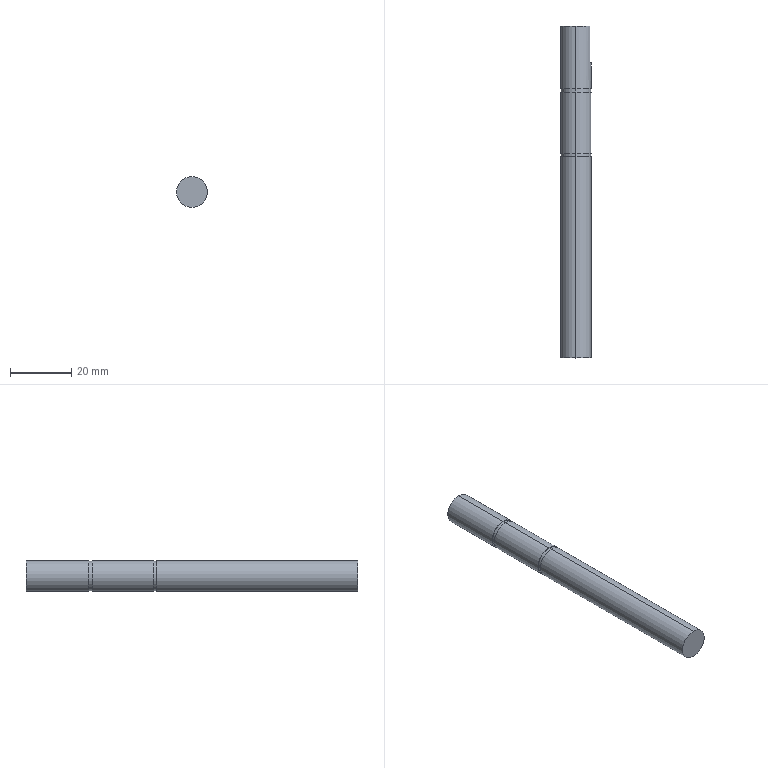Part | NX | features BREP 1 | 1 solid | 18 faces | box 10 x 108 x 10 mm | volume 8451 mm3 | cylinder 10 | plane 8 | commonest cylinder face diameters 10 x6 9.6 x4
STEP:
#1=CARTESIAN_POINT('',(0.,65.4,5.));
#2=VERTEX_POINT('',#1);
#3=CARTESIAN_POINT('',(0.,65.4,-5.));
#4=VERTEX_POINT('',#3);
#5=CARTESIAN_POINT('',(0.,65.4,0.));
#6=DIRECTION('',(0.,1.,0.));
#7=DIRECTION('',(0.,0.,1.));
#8=AXIS2_PLACEMENT_3D('',#5,#6,#7);
#9=CIRCLE('',#8,5.);
#10=EDGE_CURVE('',#2,#4,#9,.T.);
#11=ORIENTED_EDGE('',*,*,#10,.F.);
#12=CARTESIAN_POINT('',(0.,0.,5.));
#13=VERTEX_POINT('',#12);
#14=CARTESIAN_POINT('',(0.,-32.611,5.));
#15=DIRECTION('',(0.,-1.,0.));
#16=VECTOR('',#15,1000.);
#17=LINE('',#14,#16);
#18=EDGE_CURVE('',#13,#2,#17,.F.);
#19=ORIENTED_EDGE('',*,*,#18,.F.);
#20=CARTESIAN_POINT('',(0.,0.,-5.));
#21=VERTEX_POINT('',#20);
#22=CARTESIAN_POINT('',(0.,0.,0.));
#23=DIRECTION('',(0.,-1.,0.));
#24=DIRECTION('',(0.,0.,-1.));
#25=AXIS2_PLACEMENT_3D('',#22,#23,#24);
#26=CIRCLE('',#25,5.);
#27=EDGE_CURVE('',#21,#13,#26,.T.);
#28=ORIENTED_EDGE('',*,*,#27,.F.);
#29=CARTESIAN_POINT('',(0.,-32.611,-5.));
#30=DIRECTION('',(0.,-1.,0.));
#31=VECTOR('',#30,1000.);
#32=LINE('',#29,#31);
#33=EDGE_CURVE('',#21,#4,#32,.F.);
#34=ORIENTED_EDGE('',*,*,#33,.T.);
#35=EDGE_LOOP('',(#11,#19,#28,#34));
#36=FACE_BOUND('',#35,.T.);
#37=CARTESIAN_POINT('',(0.,-32.611,0.));
#38=DIRECTION('',(0.,-1.,0.));
#39=DIRECTION('',(0.,0.,1.));
#40=AXIS2_PLACEMENT_3D('',#37,#38,#39);
#41=CYLINDRICAL_SURFACE('',#40,5.);
#42=ADVANCED_FACE('',(#36),#41,.T.);
#43=CARTESIAN_POINT('',(0.,66.5,4.8));
#44=VERTEX_POINT('',#43);
#45=CARTESIAN_POINT('',(0.,66.5,-4.8));
#46=VERTEX_POINT('',#45);
#47=CARTESIAN_POINT('',(0.,66.5,0.));
#48=DIRECTION('',(0.,1.,0.));
#49=DIRECTION('',(0.,0.,1.));
#50=AXIS2_PLACEMENT_3D('',#47,#48,#49);
#51=CIRCLE('',#50,4.8);
#52=EDGE_CURVE('',#44,#46,#51,.T.);
#53=ORIENTED_EDGE('',*,*,#52,.F.);
#54=CARTESIAN_POINT('',(0.,65.4,4.8));
#55=VERTEX_POINT('',#54);
#56=CARTESIAN_POINT('',(0.,66.5,4.8));
#57=DIRECTION('',(0.,-1.,0.));
#58=VECTOR('',#57,1000.);
#59=LINE('',#56,#58);
#60=EDGE_CURVE('',#55,#44,#59,.F.);
#61=ORIENTED_EDGE('',*,*,#60,.F.);
#62=CARTESIAN_POINT('',(0.,65.4,-4.8));
#63=VERTEX_POINT('',#62);
#64=CARTESIAN_POINT('',(0.,65.4,0.));
#65=DIRECTION('',(0.,1.,0.));
#66=DIRECTION('',(0.,0.,1.));
#67=AXIS2_PLACEMENT_3D('',#64,#65,#66);
#68=CIRCLE('',#67,4.8);
#69=EDGE_CURVE('',#55,#63,#68,.T.);
#70=ORIENTED_EDGE('',*,*,#69,.T.);
#71=CARTESIAN_POINT('',(0.,66.5,-4.8));
#72=DIRECTION('',(0.,-1.,0.));
#73=VECTOR('',#72,1000.);
#74=LINE('',#71,#73);
#75=EDGE_CURVE('',#63,#46,#74,.F.);
#76=ORIENTED_EDGE('',*,*,#75,.T.);
#77=EDGE_LOOP('',(#53,#61,#70,#76));
#78=FACE_BOUND('',#77,.T.);
#79=CARTESIAN_POINT('',(0.,66.5,0.));
#80=DIRECTION('',(0.,-1.,0.));
#81=DIRECTION('',(0.,0.,1.));
#82=AXIS2_PLACEMENT_3D('',#79,#80,#81);
#83=CYLINDRICAL_SURFACE('',#82,4.8);
#84=ADVANCED_FACE('',(#78),#83,.T.);
#85=CARTESIAN_POINT('',(0.,86.5,5.));
#86=VERTEX_POINT('',#85);
#87=CARTESIAN_POINT('',(0.,86.5,-5.));
#88=VERTEX_POINT('',#87);
#89=CARTESIAN_POINT('',(0.,86.5,0.));
#90=DIRECTION('',(0.,1.,0.));
#91=DIRECTION('',(0.,0.,1.));
#92=AXIS2_PLACEMENT_3D('',#89,#90,#91);
#93=CIRCLE('',#92,5.);
#94=EDGE_CURVE('',#86,#88,#93,.T.);
#95=ORIENTED_EDGE('',*,*,#94,.F.);
#96=CARTESIAN_POINT('',(0.,66.5,5.));
#97=VERTEX_POINT('',#96);
#98=CARTESIAN_POINT('',(0.,-32.611,5.));
#99=DIRECTION('',(0.,-1.,0.));
#100=VECTOR('',#99,1000.);
#101=LINE('',#98,#100);
#102=EDGE_CURVE('',#97,#86,#101,.F.);
#103=ORIENTED_EDGE('',*,*,#102,.F.);
#104=CARTESIAN_POINT('',(0.,66.5,-5.));
#105=VERTEX_POINT('',#104);
#106=CARTESIAN_POINT('',(0.,66.5,0.));
#107=DIRECTION('',(0.,1.,0.));
#108=DIRECTION('',(0.,0.,1.));
#109=AXIS2_PLACEMENT_3D('',#106,#107,#108);
#110=CIRCLE('',#109,5.);
#111=EDGE_CURVE('',#97,#105,#110,.T.);
#112=ORIENTED_EDGE('',*,*,#111,.T.);
#113=CARTESIAN_POINT('',(0.,-32.611,-5.));
#114=DIRECTION('',(0.,-1.,0.));
#115=VECTOR('',#114,1000.);
#116=LINE('',#113,#115);
#117=EDGE_CURVE('',#105,#88,#116,.F.);
#118=ORIENTED_EDGE('',*,*,#117,.T.);
#119=EDGE_LOOP('',(#95,#103,#112,#118));
#120=FACE_BOUND('',#119,.T.);
#121=CARTESIAN_POINT('',(0.,-32.611,0.));
#122=DIRECTION('',(0.,-1.,0.));
#123=DIRECTION('',(0.,0.,1.));
#124=AXIS2_PLACEMENT_3D('',#121,#122,#123);
#125=CYLINDRICAL_SURFACE('',#124,5.);
#126=ADVANCED_FACE('',(#120),#125,.T.);
#127=CARTESIAN_POINT('',(0.,87.6,4.8));
#128=VERTEX_POINT('',#127);
#129=CARTESIAN_POINT('',(0.,87.6,-4.8));
#130=VERTEX_POINT('',#129);
#131=CARTESIAN_POINT('',(0.,87.6,0.));
#132=DIRECTION('',(0.,1.,0.));
#133=DIRECTION('',(0.,0.,1.));
#134=AXIS2_PLACEMENT_3D('',#131,#132,#133);
#135=CIRCLE('',#134,4.8);
#136=EDGE_CURVE('',#128,#130,#135,.T.);
#137=ORIENTED_EDGE('',*,*,#136,.F.);
#138=CARTESIAN_POINT('',(0.,86.5,4.8));
#139=VERTEX_POINT('',#138);
#140=CARTESIAN_POINT('',(0.,87.6,4.8));
#141=DIRECTION('',(0.,-1.,0.));
#142=VECTOR('',#141,1000.);
#143=LINE('',#140,#142);
#144=EDGE_CURVE('',#139,#128,#143,.F.);
#145=ORIENTED_EDGE('',*,*,#144,.F.);
#146=CARTESIAN_POINT('',(0.,86.5,-4.8));
#147=VERTEX_POINT('',#146);
#148=CARTESIAN_POINT('',(0.,86.5,0.));
#149=DIRECTION('',(0.,1.,0.));
#150=DIRECTION('',(0.,0.,1.));
#151=AXIS2_PLACEMENT_3D('',#148,#149,#150);
#152=CIRCLE('',#151,4.8);
#153=EDGE_CURVE('',#139,#147,#152,.T.);
#154=ORIENTED_EDGE('',*,*,#153,.T.);
#155=CARTESIAN_POINT('',(0.,87.6,-4.8));
#156=DIRECTION('',(0.,-1.,0.));
#157=VECTOR('',#156,1000.);
#158=LINE('',#155,#157);
#159=EDGE_CURVE('',#147,#130,#158,.F.);
#160=ORIENTED_EDGE('',*,*,#159,.T.);
#161=EDGE_LOOP('',(#137,#145,#154,#160));
#162=FACE_BOUND('',#161,.T.);
#163=CARTESIAN_POINT('',(0.,87.6,0.));
#164=DIRECTION('',(0.,-1.,0.));
#165=DIRECTION('',(0.,0.,1.));
#166=AXIS2_PLACEMENT_3D('',#163,#164,#165);
#167=CYLINDRICAL_SURFACE('',#166,4.8);
#168=ADVANCED_FACE('',(#162),#167,.T.);
#169=CARTESIAN_POINT('',(4.5,108.,2.179));
#170=VERTEX_POINT('',#169);
#171=CARTESIAN_POINT('',(0.,108.,5.));
#172=VERTEX_POINT('',#171);
#173=CARTESIAN_POINT('',(0.,108.,0.));
#174=DIRECTION('',(0.,-1.,0.));
#175=DIRECTION('',(0.,0.,-1.));
#176=AXIS2_PLACEMENT_3D('',#173,#174,#175);
#177=CIRCLE('',#176,5.);
#178=EDGE_CURVE('',#170,#172,#177,.T.);
#179=ORIENTED_EDGE('',*,*,#178,.T.);
#180=CARTESIAN_POINT('',(0.,87.6,5.));
#181=VERTEX_POINT('',#180);
#182=CARTESIAN_POINT('',(0.,-32.611,5.));
#183=DIRECTION('',(0.,-1.,0.));
#184=VECTOR('',#183,1000.);
#185=LINE('',#182,#184);
#186=EDGE_CURVE('',#181,#172,#185,.F.);
#187=ORIENTED_EDGE('',*,*,#186,.F.);
#188=CARTESIAN_POINT('',(0.,87.6,-5.));
#189=VERTEX_POINT('',#188);
#190=CARTESIAN_POINT('',(0.,87.6,0.));
#191=DIRECTION('',(0.,1.,0.));
#192=DIRECTION('',(0.,0.,1.));
#193=AXIS2_PLACEMENT_3D('',#190,#191,#192);
#194=CIRCLE('',#193,5.);
#195=EDGE_CURVE('',#181,#189,#194,.T.);
#196=ORIENTED_EDGE('',*,*,#195,.T.);
#197=CARTESIAN_POINT('',(0.,108.,-5.));
#198=VERTEX_POINT('',#197);
#199=CARTESIAN_POINT('',(0.,-32.611,-5.));
#200=DIRECTION('',(0.,-1.,0.));
#201=VECTOR('',#200,1000.);
#202=LINE('',#199,#201);
#203=EDGE_CURVE('',#189,#198,#202,.F.);
#204=ORIENTED_EDGE('',*,*,#203,.T.);
#205=CARTESIAN_POINT('',(4.5,108.,-2.179));
#206=VERTEX_POINT('',#205);
#207=CARTESIAN_POINT('',(0.,108.,0.));
#208=DIRECTION('',(0.,-1.,0.));
#209=DIRECTION('',(0.,0.,-1.));
#210=AXIS2_PLACEMENT_3D('',#207,#208,#209);
#211=CIRCLE('',#210,5.);
#212=EDGE_CURVE('',#198,#206,#211,.T.);
#213=ORIENTED_EDGE('',*,*,#212,.T.);
#214=CARTESIAN_POINT('',(4.5,96.,-2.179));
#215=VERTEX_POINT('',#214);
#216=CARTESIAN_POINT('',(4.5,-32.611,-2.179));
#217=DIRECTION('',(0.,1.,0.));
#218=VECTOR('',#217,1000.);
#219=LINE('',#216,#218);
#220=EDGE_CURVE('',#215,#206,#219,.T.);
#221=ORIENTED_EDGE('',*,*,#220,.F.);
#222=CARTESIAN_POINT('',(4.5,96.,2.179));
#223=VERTEX_POINT('',#222);
#224=CARTESIAN_POINT('',(0.,96.,0.));
#225=DIRECTION('',(0.,1.,0.));
#226=DIRECTION('',(0.,0.,-1.));
#227=AXIS2_PLACEMENT_3D('',#224,#225,#226);
#228=CIRCLE('',#227,5.);
#229=EDGE_CURVE('',#223,#215,#228,.T.);
#230=ORIENTED_EDGE('',*,*,#229,.F.);
#231=CARTESIAN_POINT('',(4.5,-32.611,2.179));
#232=DIRECTION('',(0.,-1.,0.));
#233=VECTOR('',#232,1000.);
#234=LINE('',#231,#233);
#235=EDGE_CURVE('',#170,#223,#234,.T.);
#236=ORIENTED_EDGE('',*,*,#235,.F.);
#237=EDGE_LOOP('',(#179,#187,#196,#204,#213,#221,#230,#236));
#238=FACE_BOUND('',#237,.T.);
#239=CARTESIAN_POINT('',(0.,-32.611,0.));
#240=DIRECTION('',(0.,-1.,0.));
#241=DIRECTION('',(0.,0.,1.));
#242=AXIS2_PLACEMENT_3D('',#239,#240,#241);
#243=CYLINDRICAL_SURFACE('',#242,5.);
#244=ADVANCED_FACE('',(#238),#243,.T.);
#245=CARTESIAN_POINT('',(4.5,108.,-5.));
#246=DIRECTION('',(0.,0.,1.));
#247=VECTOR('',#246,1000.);
#248=LINE('',#245,#247);
#249=EDGE_CURVE('',#206,#170,#248,.T.);
#250=ORIENTED_EDGE('',*,*,#249,.F.);
#251=ORIENTED_EDGE('',*,*,#212,.F.);
#252=CARTESIAN_POINT('',(0.,108.,0.));
#253=DIRECTION('',(0.,-1.,0.));
#254=DIRECTION('',(0.,0.,-1.));
#255=AXIS2_PLACEMENT_3D('',#252,#253,#254);
#256=CIRCLE('',#255,5.);
#257=EDGE_CURVE('',#172,#198,#256,.T.);
#258=ORIENTED_EDGE('',*,*,#257,.F.);
#259=ORIENTED_EDGE('',*,*,#178,.F.);
#260=EDGE_LOOP('',(#250,#251,#258,#259));
#261=FACE_BOUND('',#260,.T.);
#262=CARTESIAN_POINT('',(0.,108.,0.));
#263=DIRECTION('',(0.,1.,0.));
#264=DIRECTION('',(0.,0.,-1.));
#265=AXIS2_PLACEMENT_3D('',#262,#263,#264);
#266=PLANE('',#265);
#267=ADVANCED_FACE('',(#261),#266,.T.);
#268=ORIENTED_EDGE('',*,*,#186,.T.);
#269=ORIENTED_EDGE('',*,*,#257,.T.);
#270=ORIENTED_EDGE('',*,*,#203,.F.);
#271=CARTESIAN_POINT('',(0.,87.6,0.));
#272=DIRECTION('',(0.,1.,0.));
#273=DIRECTION('',(0.,0.,1.));
#274=AXIS2_PLACEMENT_3D('',#271,#272,#273);
#275=CIRCLE('',#274,5.);
#276=EDGE_CURVE('',#189,#181,#275,.T.);
#277=ORIENTED_EDGE('',*,*,#276,.T.);
#278=EDGE_LOOP('',(#268,#269,#270,#277));
#279=FACE_BOUND('',#278,.T.);
#280=CARTESIAN_POINT('',(0.,-32.611,0.));
#281=DIRECTION('',(0.,-1.,0.));
#282=DIRECTION('',(0.,0.,1.));
#283=AXIS2_PLACEMENT_3D('',#280,#281,#282);
#284=CYLINDRICAL_SURFACE('',#283,5.);
#285=ADVANCED_FACE('',(#279),#284,.T.);
#286=ORIENTED_EDGE('',*,*,#229,.T.);
#287=CARTESIAN_POINT('',(4.5,96.,-5.));
#288=DIRECTION('',(0.,0.,1.));
#289=VECTOR('',#288,1000.);
#290=LINE('',#287,#289);
#291=EDGE_CURVE('',#215,#223,#290,.T.);
#292=ORIENTED_EDGE('',*,*,#291,.T.);
#293=EDGE_LOOP('',(#286,#292));
#294=FACE_BOUND('',#293,.T.);
#295=CARTESIAN_POINT('',(4.5,96.,-5.));
#296=DIRECTION('',(0.,-1.,0.));
#297=DIRECTION('',(0.,0.,1.));
#298=AXIS2_PLACEMENT_3D('',#295,#296,#297);
#299=PLANE('',#298);
#300=ADVANCED_FACE('',(#294),#299,.F.);
#301=ORIENTED_EDGE('',*,*,#220,.T.);
#302=ORIENTED_EDGE('',*,*,#249,.T.);
#303=ORIENTED_EDGE('',*,*,#235,.T.);
#304=ORIENTED_EDGE('',*,*,#291,.F.);
#305=EDGE_LOOP('',(#301,#302,#303,#304));
#306=FACE_BOUND('',#305,.T.);
#307=CARTESIAN_POINT('',(4.5,108.,-5.));
#308=DIRECTION('',(-1.,0.,0.));
#309=DIRECTION('',(0.,1.,0.));
#310=AXIS2_PLACEMENT_3D('',#307,#308,#309);
#311=PLANE('',#310);
#312=ADVANCED_FACE('',(#306),#311,.F.);
#313=ORIENTED_EDGE('',*,*,#276,.F.);
#314=ORIENTED_EDGE('',*,*,#195,.F.);
#315=EDGE_LOOP('',(#313,#314));
#316=FACE_BOUND('',#315,.T.);
#317=CARTESIAN_POINT('',(0.,87.6,0.));
#318=DIRECTION('',(0.,1.,0.));
#319=DIRECTION('',(0.,0.,1.));
#320=AXIS2_PLACEMENT_3D('',#317,#318,#319);
#321=CIRCLE('',#320,4.8);
#322=EDGE_CURVE('',#130,#128,#321,.T.);
#323=ORIENTED_EDGE('',*,*,#322,.T.);
#324=ORIENTED_EDGE('',*,*,#136,.T.);
#325=EDGE_LOOP('',(#323,#324));
#326=FACE_BOUND('',#325,.T.);
#327=CARTESIAN_POINT('',(0.,87.6,0.));
#328=DIRECTION('',(0.,1.,0.));
#329=DIRECTION('',(0.,0.,-1.));
#330=AXIS2_PLACEMENT_3D('',#327,#328,#329);
#331=PLANE('',#330);
#332=ADVANCED_FACE('',(#316,#326),#331,.F.);
#333=CARTESIAN_POINT('',(0.,86.5,0.));
#334=DIRECTION('',(0.,1.,0.));
#335=DIRECTION('',(0.,0.,1.));
#336=AXIS2_PLACEMENT_3D('',#333,#334,#335);
#337=CIRCLE('',#336,5.);
#338=EDGE_CURVE('',#88,#86,#337,.T.);
#339=ORIENTED_EDGE('',*,*,#338,.T.);
#340=ORIENTED_EDGE('',*,*,#94,.T.);
#341=EDGE_LOOP('',(#339,#340));
#342=FACE_BOUND('',#341,.T.);
#343=CARTESIAN_POINT('',(0.,86.5,0.));
#344=DIRECTION('',(0.,1.,0.));
#345=DIRECTION('',(0.,0.,1.));
#346=AXIS2_PLACEMENT_3D('',#343,#344,#345);
#347=CIRCLE('',#346,4.8);
#348=EDGE_CURVE('',#147,#139,#347,.T.);
#349=ORIENTED_EDGE('',*,*,#348,.F.);
#350=ORIENTED_EDGE('',*,*,#153,.F.);
#351=EDGE_LOOP('',(#349,#350));
#352=FACE_BOUND('',#351,.T.);
#353=CARTESIAN_POINT('',(0.,86.5,0.));
#354=DIRECTION('',(0.,1.,0.));
#355=DIRECTION('',(0.,0.,-1.));
#356=AXIS2_PLACEMENT_3D('',#353,#354,#355);
#357=PLANE('',#356);
#358=ADVANCED_FACE('',(#342,#352),#357,.T.);
#359=ORIENTED_EDGE('',*,*,#144,.T.);
#360=ORIENTED_EDGE('',*,*,#322,.F.);
#361=ORIENTED_EDGE('',*,*,#159,.F.);
#362=ORIENTED_EDGE('',*,*,#348,.T.);
#363=EDGE_LOOP('',(#359,#360,#361,#362));
#364=FACE_BOUND('',#363,.T.);
#365=CARTESIAN_POINT('',(0.,87.6,0.));
#366=DIRECTION('',(0.,-1.,0.));
#367=DIRECTION('',(0.,0.,1.));
#368=AXIS2_PLACEMENT_3D('',#365,#366,#367);
#369=CYLINDRICAL_SURFACE('',#368,4.8);
#370=ADVANCED_FACE('',(#364),#369,.T.);
#371=ORIENTED_EDGE('',*,*,#102,.T.);
#372=ORIENTED_EDGE('',*,*,#338,.F.);
#373=ORIENTED_EDGE('',*,*,#117,.F.);
#374=CARTESIAN_POINT('',(0.,66.5,0.));
#375=DIRECTION('',(0.,1.,0.));
#376=DIRECTION('',(0.,0.,1.));
#377=AXIS2_PLACEMENT_3D('',#374,#375,#376);
#378=CIRCLE('',#377,5.);
#379=EDGE_CURVE('',#105,#97,#378,.T.);
#380=ORIENTED_EDGE('',*,*,#379,.T.);
#381=EDGE_LOOP('',(#371,#372,#373,#380));
#382=FACE_BOUND('',#381,.T.);
#383=CARTESIAN_POINT('',(0.,-32.611,0.));
#384=DIRECTION('',(0.,-1.,0.));
#385=DIRECTION('',(0.,0.,1.));
#386=AXIS2_PLACEMENT_3D('',#383,#384,#385);
#387=CYLINDRICAL_SURFACE('',#386,5.);
#388=ADVANCED_FACE('',(#382),#387,.T.);
#389=ORIENTED_EDGE('',*,*,#379,.F.);
#390=ORIENTED_EDGE('',*,*,#111,.F.);
#391=EDGE_LOOP('',(#389,#390));
#392=FACE_BOUND('',#391,.T.);
#393=CARTESIAN_POINT('',(0.,66.5,0.));
#394=DIRECTION('',(0.,1.,0.));
#395=DIRECTION('',(0.,0.,1.));
#396=AXIS2_PLACEMENT_3D('',#393,#394,#395);
#397=CIRCLE('',#396,4.8);
#398=EDGE_CURVE('',#46,#44,#397,.T.);
#399=ORIENTED_EDGE('',*,*,#398,.T.);
#400=ORIENTED_EDGE('',*,*,#52,.T.);
#401=EDGE_LOOP('',(#399,#400));
#402=FACE_BOUND('',#401,.T.);
#403=CARTESIAN_POINT('',(0.,66.5,0.));
#404=DIRECTION('',(0.,1.,0.));
#405=DIRECTION('',(0.,0.,-1.));
#406=AXIS2_PLACEMENT_3D('',#403,#404,#405);
#407=PLANE('',#406);
#408=ADVANCED_FACE('',(#392,#402),#407,.F.);
#409=CARTESIAN_POINT('',(0.,65.4,0.));
#410=DIRECTION('',(0.,1.,0.));
#411=DIRECTION('',(0.,0.,1.));
#412=AXIS2_PLACEMENT_3D('',#409,#410,#411);
#413=CIRCLE('',#412,5.);
#414=EDGE_CURVE('',#4,#2,#413,.T.);
#415=ORIENTED_EDGE('',*,*,#414,.T.);
#416=ORIENTED_EDGE('',*,*,#10,.T.);
#417=EDGE_LOOP('',(#415,#416));
#418=FACE_BOUND('',#417,.T.);
#419=CARTESIAN_POINT('',(0.,65.4,0.));
#420=DIRECTION('',(0.,1.,0.));
#421=DIRECTION('',(0.,0.,1.));
#422=AXIS2_PLACEMENT_3D('',#419,#420,#421);
#423=CIRCLE('',#422,4.8);
#424=EDGE_CURVE('',#63,#55,#423,.T.);
#425=ORIENTED_EDGE('',*,*,#424,.F.);
#426=ORIENTED_EDGE('',*,*,#69,.F.);
#427=EDGE_LOOP('',(#425,#426));
#428=FACE_BOUND('',#427,.T.);
#429=CARTESIAN_POINT('',(0.,65.4,0.));
#430=DIRECTION('',(0.,1.,0.));
#431=DIRECTION('',(0.,0.,-1.));
#432=AXIS2_PLACEMENT_3D('',#429,#430,#431);
#433=PLANE('',#432);
#434=ADVANCED_FACE('',(#418,#428),#433,.T.);
#435=ORIENTED_EDGE('',*,*,#60,.T.);
#436=ORIENTED_EDGE('',*,*,#398,.F.);
#437=ORIENTED_EDGE('',*,*,#75,.F.);
#438=ORIENTED_EDGE('',*,*,#424,.T.);
#439=EDGE_LOOP('',(#435,#436,#437,#438));
#440=FACE_BOUND('',#439,.T.);
#441=CARTESIAN_POINT('',(0.,66.5,0.));
#442=DIRECTION('',(0.,-1.,0.));
#443=DIRECTION('',(0.,0.,1.));
#444=AXIS2_PLACEMENT_3D('',#441,#442,#443);
#445=CYLINDRICAL_SURFACE('',#444,4.8);
#446=ADVANCED_FACE('',(#440),#445,.T.);
#447=ORIENTED_EDGE('',*,*,#27,.T.);
#448=CARTESIAN_POINT('',(0.,0.,0.));
#449=DIRECTION('',(0.,-1.,0.));
#450=DIRECTION('',(0.,0.,-1.));
#451=AXIS2_PLACEMENT_3D('',#448,#449,#450);
#452=CIRCLE('',#451,5.);
#453=EDGE_CURVE('',#13,#21,#452,.T.);
#454=ORIENTED_EDGE('',*,*,#453,.T.);
#455=EDGE_LOOP('',(#447,#454));
#456=FACE_BOUND('',#455,.T.);
#457=CARTESIAN_POINT('',(5.,0.,0.));
#458=DIRECTION('',(0.,-1.,0.));
#459=DIRECTION('',(0.,0.,1.));
#460=AXIS2_PLACEMENT_3D('',#457,#458,#459);
#461=PLANE('',#460);
#462=ADVANCED_FACE('',(#456),#461,.T.);
#463=ORIENTED_EDGE('',*,*,#18,.T.);
#464=ORIENTED_EDGE('',*,*,#414,.F.);
#465=ORIENTED_EDGE('',*,*,#33,.F.);
#466=ORIENTED_EDGE('',*,*,#453,.F.);
#467=EDGE_LOOP('',(#463,#464,#465,#466));
#468=FACE_BOUND('',#467,.T.);
#469=CARTESIAN_POINT('',(0.,-32.611,0.));
#470=DIRECTION('',(0.,-1.,0.));
#471=DIRECTION('',(0.,0.,1.));
#472=AXIS2_PLACEMENT_3D('',#469,#470,#471);
#473=CYLINDRICAL_SURFACE('',#472,5.);
#474=ADVANCED_FACE('',(#468),#473,.T.);
#475=CLOSED_SHELL('',(#42,#84,#126,#168,#244,#267,#285,#300,#312,#332,#358,#370,#388,#408,#434,#446,#462,#474));
#476=MANIFOLD_SOLID_BREP('',#475);
#477=(LENGTH_UNIT()NAMED_UNIT(*)SI_UNIT(.MILLI.,.METRE.));
#478=UNCERTAINTY_MEASURE_WITH_UNIT(LENGTH_MEASURE(0.00001),#477,'','');
#479=(NAMED_UNIT(*)PLANE_ANGLE_UNIT()SI_UNIT($,.RADIAN.));
#480=(NAMED_UNIT(*)SI_UNIT($,.STERADIAN.)SOLID_ANGLE_UNIT());
#481=(GEOMETRIC_REPRESENTATION_CONTEXT(3)GLOBAL_UNCERTAINTY_ASSIGNED_CONTEXT((#478))GLOBAL_UNIT_ASSIGNED_CONTEXT((#477,#479,#480))REPRESENTATION_CONTEXT('',''));
#482=ADVANCED_BREP_SHAPE_REPRESENTATION('',(#476),#481);